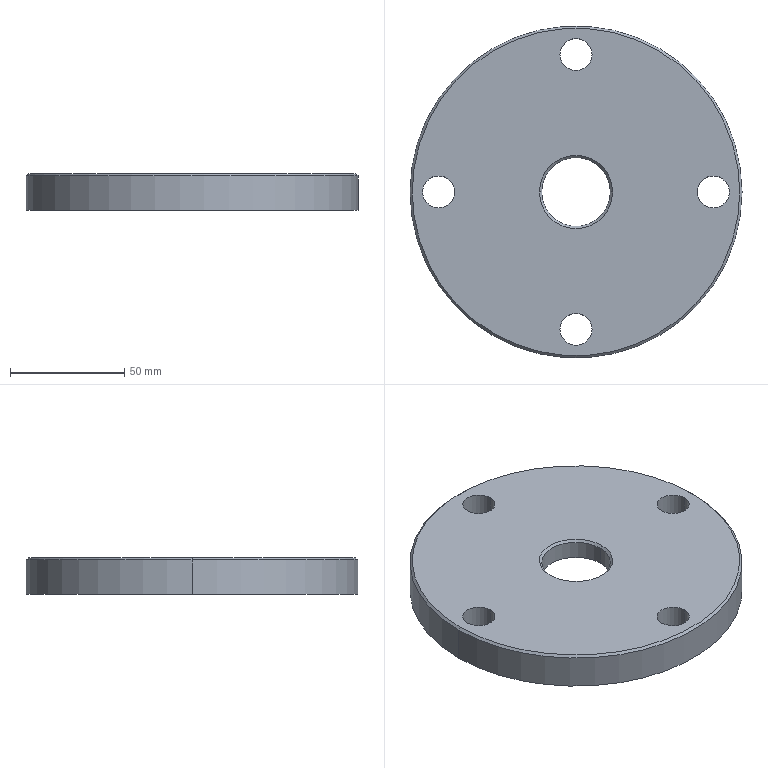Part | SolidWorks | features ICE 3, Chamfer 1, Extrusion 1 | 1 solid | 23 faces | box 145 x 145 x 16 mm | volume 201040 mm3 | cylinder 14 | cone 6 | plane 3 | commonest cylinder face diameters 14 x8 30 x2 92 x2 145 x2
STEP:
#1=CARTESIAN_POINT('',(71.5,0.,16.));
#2=VERTEX_POINT('',#1);
#3=CARTESIAN_POINT('',(-71.5,0.,16.));
#4=VERTEX_POINT('',#3);
#5=CARTESIAN_POINT('',(0.,0.,16.));
#6=DIRECTION('',(0.,0.,1.));
#7=DIRECTION('',(1.,0.,0.));
#8=AXIS2_PLACEMENT_3D('',#5,#6,#7);
#9=CIRCLE('',#8,71.5);
#10=EDGE_CURVE('',#2,#4,#9,.T.);
#11=ORIENTED_EDGE('',*,*,#10,.F.);
#12=CARTESIAN_POINT('',(72.5,0.,15.));
#13=VERTEX_POINT('',#12);
#14=CARTESIAN_POINT('',(71.5,0.,16.));
#15=DIRECTION('',(0.7071,0.,-0.7071));
#16=VECTOR('',#15,1000.);
#17=LINE('',#14,#16);
#18=EDGE_CURVE('',#2,#13,#17,.T.);
#19=ORIENTED_EDGE('',*,*,#18,.T.);
#20=CARTESIAN_POINT('',(-72.5,0.,15.));
#21=VERTEX_POINT('',#20);
#22=CARTESIAN_POINT('',(0.,0.,15.));
#23=DIRECTION('',(0.,0.,-1.));
#24=DIRECTION('',(1.,0.,0.));
#25=AXIS2_PLACEMENT_3D('',#22,#23,#24);
#26=CIRCLE('',#25,72.5);
#27=EDGE_CURVE('',#21,#13,#26,.T.);
#28=ORIENTED_EDGE('',*,*,#27,.F.);
#29=CARTESIAN_POINT('',(-71.5,0.,16.));
#30=DIRECTION('',(-0.7071,0.,-0.7071));
#31=VECTOR('',#30,1000.);
#32=LINE('',#29,#31);
#33=EDGE_CURVE('',#4,#21,#32,.T.);
#34=ORIENTED_EDGE('',*,*,#33,.F.);
#35=EDGE_LOOP('',(#11,#19,#28,#34));
#36=FACE_OUTER_BOUND('',#35,.T.);
#37=CARTESIAN_POINT('',(0.,0.,16.));
#38=DIRECTION('',(0.,0.,-1.));
#39=DIRECTION('',(-1.,0.,0.));
#40=AXIS2_PLACEMENT_3D('',#37,#38,#39);
#41=CONICAL_SURFACE('',#40,71.5,0.7854);
#42=ADVANCED_FACE('',(#36),#41,.T.);
#43=CARTESIAN_POINT('',(46.,0.,1.));
#44=VERTEX_POINT('',#43);
#45=CARTESIAN_POINT('',(-46.,0.,1.));
#46=VERTEX_POINT('',#45);
#47=CARTESIAN_POINT('',(0.,0.,1.));
#48=DIRECTION('',(0.,0.,-1.));
#49=DIRECTION('',(1.,0.,0.));
#50=AXIS2_PLACEMENT_3D('',#47,#48,#49);
#51=CIRCLE('',#50,46.);
#52=EDGE_CURVE('',#44,#46,#51,.T.);
#53=ORIENTED_EDGE('',*,*,#52,.F.);
#54=CARTESIAN_POINT('',(47.,0.,0.));
#55=VERTEX_POINT('',#54);
#56=CARTESIAN_POINT('',(46.,0.,1.));
#57=DIRECTION('',(0.7071,0.,-0.7071));
#58=VECTOR('',#57,1000.);
#59=LINE('',#56,#58);
#60=EDGE_CURVE('',#44,#55,#59,.T.);
#61=ORIENTED_EDGE('',*,*,#60,.T.);
#62=CARTESIAN_POINT('',(-47.,0.,0.));
#63=VERTEX_POINT('',#62);
#64=CARTESIAN_POINT('',(0.,0.,0.));
#65=DIRECTION('',(0.,0.,1.));
#66=DIRECTION('',(1.,0.,0.));
#67=AXIS2_PLACEMENT_3D('',#64,#65,#66);
#68=CIRCLE('',#67,47.);
#69=EDGE_CURVE('',#63,#55,#68,.T.);
#70=ORIENTED_EDGE('',*,*,#69,.F.);
#71=CARTESIAN_POINT('',(-46.,0.,1.));
#72=DIRECTION('',(-0.7071,0.,-0.7071));
#73=VECTOR('',#72,1000.);
#74=LINE('',#71,#73);
#75=EDGE_CURVE('',#46,#63,#74,.T.);
#76=ORIENTED_EDGE('',*,*,#75,.F.);
#77=EDGE_LOOP('',(#53,#61,#70,#76));
#78=FACE_OUTER_BOUND('',#77,.T.);
#79=CARTESIAN_POINT('',(0.,0.,1.));
#80=DIRECTION('',(0.,0.,-1.));
#81=DIRECTION('',(-1.,0.,0.));
#82=AXIS2_PLACEMENT_3D('',#79,#80,#81);
#83=CONICAL_SURFACE('',#82,46.,0.7854);
#84=ADVANCED_FACE('',(#78),#83,.F.);
#85=CARTESIAN_POINT('',(-15.,0.,15.));
#86=VERTEX_POINT('',#85);
#87=CARTESIAN_POINT('',(15.,0.,15.));
#88=VERTEX_POINT('',#87);
#89=CARTESIAN_POINT('',(0.,0.,15.));
#90=DIRECTION('',(0.,0.,1.));
#91=DIRECTION('',(1.,0.,0.));
#92=AXIS2_PLACEMENT_3D('',#89,#90,#91);
#93=CIRCLE('',#92,15.);
#94=EDGE_CURVE('',#86,#88,#93,.T.);
#95=ORIENTED_EDGE('',*,*,#94,.F.);
#96=CARTESIAN_POINT('',(-16.,0.,16.));
#97=VERTEX_POINT('',#96);
#98=CARTESIAN_POINT('',(-15.,0.,15.));
#99=DIRECTION('',(-0.7071,0.,0.7071));
#100=VECTOR('',#99,1000.);
#101=LINE('',#98,#100);
#102=EDGE_CURVE('',#86,#97,#101,.T.);
#103=ORIENTED_EDGE('',*,*,#102,.T.);
#104=CARTESIAN_POINT('',(16.,0.,16.));
#105=VERTEX_POINT('',#104);
#106=CARTESIAN_POINT('',(0.,0.,16.));
#107=DIRECTION('',(0.,0.,-1.));
#108=DIRECTION('',(1.,0.,0.));
#109=AXIS2_PLACEMENT_3D('',#106,#107,#108);
#110=CIRCLE('',#109,16.);
#111=EDGE_CURVE('',#105,#97,#110,.T.);
#112=ORIENTED_EDGE('',*,*,#111,.F.);
#113=CARTESIAN_POINT('',(15.,0.,15.));
#114=DIRECTION('',(0.7071,0.,0.7071));
#115=VECTOR('',#114,1000.);
#116=LINE('',#113,#115);
#117=EDGE_CURVE('',#88,#105,#116,.T.);
#118=ORIENTED_EDGE('',*,*,#117,.F.);
#119=EDGE_LOOP('',(#95,#103,#112,#118));
#120=FACE_OUTER_BOUND('',#119,.T.);
#121=CARTESIAN_POINT('',(0.,0.,15.));
#122=DIRECTION('',(0.,0.,1.));
#123=DIRECTION('',(1.,0.,0.));
#124=AXIS2_PLACEMENT_3D('',#121,#122,#123);
#125=CONICAL_SURFACE('',#124,15.,0.7854);
#126=ADVANCED_FACE('',(#120),#125,.F.);
#127=CARTESIAN_POINT('',(15.,0.,7.));
#128=VERTEX_POINT('',#127);
#129=CARTESIAN_POINT('',(-15.,0.,7.));
#130=VERTEX_POINT('',#129);
#131=CARTESIAN_POINT('',(0.,0.,7.));
#132=DIRECTION('',(0.,0.,-1.));
#133=DIRECTION('',(-1.,0.,0.));
#134=AXIS2_PLACEMENT_3D('',#131,#132,#133);
#135=CIRCLE('',#134,15.);
#136=EDGE_CURVE('',#128,#130,#135,.T.);
#137=ORIENTED_EDGE('',*,*,#136,.T.);
#138=CARTESIAN_POINT('',(-15.,0.,0.));
#139=DIRECTION('',(0.,0.,1.));
#140=VECTOR('',#139,1000.);
#141=LINE('',#138,#140);
#142=EDGE_CURVE('',#130,#86,#141,.T.);
#143=ORIENTED_EDGE('',*,*,#142,.T.);
#144=ORIENTED_EDGE('',*,*,#94,.T.);
#145=CARTESIAN_POINT('',(15.,0.,0.));
#146=DIRECTION('',(0.,0.,1.));
#147=VECTOR('',#146,1000.);
#148=LINE('',#145,#147);
#149=EDGE_CURVE('',#128,#88,#148,.T.);
#150=ORIENTED_EDGE('',*,*,#149,.F.);
#151=EDGE_LOOP('',(#137,#143,#144,#150));
#152=FACE_OUTER_BOUND('',#151,.T.);
#153=CARTESIAN_POINT('',(0.,0.,0.));
#154=DIRECTION('',(0.,0.,1.));
#155=DIRECTION('',(1.,0.,0.));
#156=AXIS2_PLACEMENT_3D('',#153,#154,#155);
#157=CYLINDRICAL_SURFACE('',#156,15.);
#158=ADVANCED_FACE('',(#152),#157,.F.);
#159=CARTESIAN_POINT('',(46.,0.,7.));
#160=VERTEX_POINT('',#159);
#161=CARTESIAN_POINT('',(-46.,0.,7.));
#162=VERTEX_POINT('',#161);
#163=CARTESIAN_POINT('',(0.,0.,7.));
#164=DIRECTION('',(0.,0.,-1.));
#165=DIRECTION('',(-1.,0.,0.));
#166=AXIS2_PLACEMENT_3D('',#163,#164,#165);
#167=CIRCLE('',#166,46.);
#168=EDGE_CURVE('',#160,#162,#167,.T.);
#169=ORIENTED_EDGE('',*,*,#168,.F.);
#170=CARTESIAN_POINT('',(46.,0.,7.));
#171=DIRECTION('',(0.,0.,-1.));
#172=VECTOR('',#171,1000.);
#173=LINE('',#170,#172);
#174=EDGE_CURVE('',#160,#44,#173,.T.);
#175=ORIENTED_EDGE('',*,*,#174,.T.);
#176=ORIENTED_EDGE('',*,*,#52,.T.);
#177=CARTESIAN_POINT('',(-46.,0.,7.));
#178=DIRECTION('',(0.,0.,-1.));
#179=VECTOR('',#178,1000.);
#180=LINE('',#177,#179);
#181=EDGE_CURVE('',#162,#46,#180,.T.);
#182=ORIENTED_EDGE('',*,*,#181,.F.);
#183=EDGE_LOOP('',(#169,#175,#176,#182));
#184=FACE_OUTER_BOUND('',#183,.T.);
#185=CARTESIAN_POINT('',(0.,0.,7.));
#186=DIRECTION('',(0.,0.,-1.));
#187=DIRECTION('',(-1.,0.,0.));
#188=AXIS2_PLACEMENT_3D('',#185,#186,#187);
#189=CYLINDRICAL_SURFACE('',#188,46.);
#190=ADVANCED_FACE('',(#184),#189,.F.);
#191=CARTESIAN_POINT('',(53.,0.,0.));
#192=VERTEX_POINT('',#191);
#193=CARTESIAN_POINT('',(67.,0.,0.));
#194=VERTEX_POINT('',#193);
#195=CARTESIAN_POINT('',(60.,0.,0.));
#196=DIRECTION('',(0.,0.,1.));
#197=DIRECTION('',(1.,0.,0.));
#198=AXIS2_PLACEMENT_3D('',#195,#196,#197);
#199=CIRCLE('',#198,7.);
#200=EDGE_CURVE('',#192,#194,#199,.T.);
#201=ORIENTED_EDGE('',*,*,#200,.F.);
#202=CARTESIAN_POINT('',(53.,0.,16.));
#203=VERTEX_POINT('',#202);
#204=CARTESIAN_POINT('',(53.,0.,0.));
#205=DIRECTION('',(0.,0.,1.));
#206=VECTOR('',#205,1000.);
#207=LINE('',#204,#206);
#208=EDGE_CURVE('',#192,#203,#207,.T.);
#209=ORIENTED_EDGE('',*,*,#208,.T.);
#210=CARTESIAN_POINT('',(67.,0.,16.));
#211=VERTEX_POINT('',#210);
#212=CARTESIAN_POINT('',(60.,0.,16.));
#213=DIRECTION('',(0.,0.,1.));
#214=DIRECTION('',(1.,0.,0.));
#215=AXIS2_PLACEMENT_3D('',#212,#213,#214);
#216=CIRCLE('',#215,7.);
#217=EDGE_CURVE('',#203,#211,#216,.T.);
#218=ORIENTED_EDGE('',*,*,#217,.T.);
#219=CARTESIAN_POINT('',(67.,0.,0.));
#220=DIRECTION('',(0.,0.,1.));
#221=VECTOR('',#220,1000.);
#222=LINE('',#219,#221);
#223=EDGE_CURVE('',#194,#211,#222,.T.);
#224=ORIENTED_EDGE('',*,*,#223,.F.);
#225=EDGE_LOOP('',(#201,#209,#218,#224));
#226=FACE_OUTER_BOUND('',#225,.T.);
#227=CARTESIAN_POINT('',(60.,0.,0.));
#228=DIRECTION('',(0.,0.,1.));
#229=DIRECTION('',(1.,0.,0.));
#230=AXIS2_PLACEMENT_3D('',#227,#228,#229);
#231=CYLINDRICAL_SURFACE('',#230,7.);
#232=ADVANCED_FACE('',(#226),#231,.F.);
#233=CARTESIAN_POINT('',(-7.,-60.,0.));
#234=VERTEX_POINT('',#233);
#235=CARTESIAN_POINT('',(7.,-60.,0.));
#236=VERTEX_POINT('',#235);
#237=CARTESIAN_POINT('',(0.,-60.,0.));
#238=DIRECTION('',(0.,0.,1.));
#239=DIRECTION('',(1.,0.,0.));
#240=AXIS2_PLACEMENT_3D('',#237,#238,#239);
#241=CIRCLE('',#240,7.);
#242=EDGE_CURVE('',#234,#236,#241,.T.);
#243=ORIENTED_EDGE('',*,*,#242,.F.);
#244=CARTESIAN_POINT('',(-7.,-60.,16.));
#245=VERTEX_POINT('',#244);
#246=CARTESIAN_POINT('',(-7.,-60.,0.));
#247=DIRECTION('',(0.,0.,1.));
#248=VECTOR('',#247,1000.);
#249=LINE('',#246,#248);
#250=EDGE_CURVE('',#234,#245,#249,.T.);
#251=ORIENTED_EDGE('',*,*,#250,.T.);
#252=CARTESIAN_POINT('',(7.,-60.,16.));
#253=VERTEX_POINT('',#252);
#254=CARTESIAN_POINT('',(0.,-60.,16.));
#255=DIRECTION('',(0.,0.,1.));
#256=DIRECTION('',(1.,0.,0.));
#257=AXIS2_PLACEMENT_3D('',#254,#255,#256);
#258=CIRCLE('',#257,7.);
#259=EDGE_CURVE('',#245,#253,#258,.T.);
#260=ORIENTED_EDGE('',*,*,#259,.T.);
#261=CARTESIAN_POINT('',(7.,-60.,0.));
#262=DIRECTION('',(0.,0.,1.));
#263=VECTOR('',#262,1000.);
#264=LINE('',#261,#263);
#265=EDGE_CURVE('',#236,#253,#264,.T.);
#266=ORIENTED_EDGE('',*,*,#265,.F.);
#267=EDGE_LOOP('',(#243,#251,#260,#266));
#268=FACE_OUTER_BOUND('',#267,.T.);
#269=CARTESIAN_POINT('',(0.,-60.,0.));
#270=DIRECTION('',(0.,0.,1.));
#271=DIRECTION('',(1.,0.,0.));
#272=AXIS2_PLACEMENT_3D('',#269,#270,#271);
#273=CYLINDRICAL_SURFACE('',#272,7.);
#274=ADVANCED_FACE('',(#268),#273,.F.);
#275=CARTESIAN_POINT('',(-67.,0.,0.));
#276=VERTEX_POINT('',#275);
#277=CARTESIAN_POINT('',(-53.,0.,0.));
#278=VERTEX_POINT('',#277);
#279=CARTESIAN_POINT('',(-60.,0.,0.));
#280=DIRECTION('',(0.,0.,1.));
#281=DIRECTION('',(1.,0.,0.));
#282=AXIS2_PLACEMENT_3D('',#279,#280,#281);
#283=CIRCLE('',#282,7.);
#284=EDGE_CURVE('',#276,#278,#283,.T.);
#285=ORIENTED_EDGE('',*,*,#284,.F.);
#286=CARTESIAN_POINT('',(-67.,0.,16.));
#287=VERTEX_POINT('',#286);
#288=CARTESIAN_POINT('',(-67.,0.,0.));
#289=DIRECTION('',(0.,0.,1.));
#290=VECTOR('',#289,1000.);
#291=LINE('',#288,#290);
#292=EDGE_CURVE('',#276,#287,#291,.T.);
#293=ORIENTED_EDGE('',*,*,#292,.T.);
#294=CARTESIAN_POINT('',(-53.,0.,16.));
#295=VERTEX_POINT('',#294);
#296=CARTESIAN_POINT('',(-60.,0.,16.));
#297=DIRECTION('',(0.,0.,1.));
#298=DIRECTION('',(1.,0.,0.));
#299=AXIS2_PLACEMENT_3D('',#296,#297,#298);
#300=CIRCLE('',#299,7.);
#301=EDGE_CURVE('',#287,#295,#300,.T.);
#302=ORIENTED_EDGE('',*,*,#301,.T.);
#303=CARTESIAN_POINT('',(-53.,0.,0.));
#304=DIRECTION('',(0.,0.,1.));
#305=VECTOR('',#304,1000.);
#306=LINE('',#303,#305);
#307=EDGE_CURVE('',#278,#295,#306,.T.);
#308=ORIENTED_EDGE('',*,*,#307,.F.);
#309=EDGE_LOOP('',(#285,#293,#302,#308));
#310=FACE_OUTER_BOUND('',#309,.T.);
#311=CARTESIAN_POINT('',(-60.,0.,0.));
#312=DIRECTION('',(0.,0.,1.));
#313=DIRECTION('',(1.,0.,0.));
#314=AXIS2_PLACEMENT_3D('',#311,#312,#313);
#315=CYLINDRICAL_SURFACE('',#314,7.);
#316=ADVANCED_FACE('',(#310),#315,.F.);
#317=CARTESIAN_POINT('',(-7.,60.,0.));
#318=VERTEX_POINT('',#317);
#319=CARTESIAN_POINT('',(7.,60.,0.));
#320=VERTEX_POINT('',#319);
#321=CARTESIAN_POINT('',(0.,60.,0.));
#322=DIRECTION('',(0.,0.,1.));
#323=DIRECTION('',(1.,0.,0.));
#324=AXIS2_PLACEMENT_3D('',#321,#322,#323);
#325=CIRCLE('',#324,7.);
#326=EDGE_CURVE('',#318,#320,#325,.T.);
#327=ORIENTED_EDGE('',*,*,#326,.F.);
#328=CARTESIAN_POINT('',(-7.,60.,16.));
#329=VERTEX_POINT('',#328);
#330=CARTESIAN_POINT('',(-7.,60.,0.));
#331=DIRECTION('',(0.,0.,1.));
#332=VECTOR('',#331,1000.);
#333=LINE('',#330,#332);
#334=EDGE_CURVE('',#318,#329,#333,.T.);
#335=ORIENTED_EDGE('',*,*,#334,.T.);
#336=CARTESIAN_POINT('',(7.,60.,16.));
#337=VERTEX_POINT('',#336);
#338=CARTESIAN_POINT('',(0.,60.,16.));
#339=DIRECTION('',(0.,0.,1.));
#340=DIRECTION('',(1.,0.,0.));
#341=AXIS2_PLACEMENT_3D('',#338,#339,#340);
#342=CIRCLE('',#341,7.);
#343=EDGE_CURVE('',#329,#337,#342,.T.);
#344=ORIENTED_EDGE('',*,*,#343,.T.);
#345=CARTESIAN_POINT('',(7.,60.,0.));
#346=DIRECTION('',(0.,0.,1.));
#347=VECTOR('',#346,1000.);
#348=LINE('',#345,#347);
#349=EDGE_CURVE('',#320,#337,#348,.T.);
#350=ORIENTED_EDGE('',*,*,#349,.F.);
#351=EDGE_LOOP('',(#327,#335,#344,#350));
#352=FACE_OUTER_BOUND('',#351,.T.);
#353=CARTESIAN_POINT('',(0.,60.,0.));
#354=DIRECTION('',(0.,0.,1.));
#355=DIRECTION('',(1.,0.,0.));
#356=AXIS2_PLACEMENT_3D('',#353,#354,#355);
#357=CYLINDRICAL_SURFACE('',#356,7.);
#358=ADVANCED_FACE('',(#352),#357,.F.);
#359=ORIENTED_EDGE('',*,*,#27,.T.);
#360=CARTESIAN_POINT('',(72.5,0.,0.));
#361=VERTEX_POINT('',#360);
#362=CARTESIAN_POINT('',(72.5,0.,16.));
#363=DIRECTION('',(0.,0.,-1.));
#364=VECTOR('',#363,1000.);
#365=LINE('',#362,#364);
#366=EDGE_CURVE('',#13,#361,#365,.T.);
#367=ORIENTED_EDGE('',*,*,#366,.T.);
#368=CARTESIAN_POINT('',(-72.5,0.,0.));
#369=VERTEX_POINT('',#368);
#370=CARTESIAN_POINT('',(0.,0.,0.));
#371=DIRECTION('',(0.,0.,1.));
#372=DIRECTION('',(1.,0.,0.));
#373=AXIS2_PLACEMENT_3D('',#370,#371,#372);
#374=CIRCLE('',#373,72.5);
#375=EDGE_CURVE('',#361,#369,#374,.T.);
#376=ORIENTED_EDGE('',*,*,#375,.T.);
#377=CARTESIAN_POINT('',(-72.5,0.,16.));
#378=DIRECTION('',(0.,0.,-1.));
#379=VECTOR('',#378,1000.);
#380=LINE('',#377,#379);
#381=EDGE_CURVE('',#21,#369,#380,.T.);
#382=ORIENTED_EDGE('',*,*,#381,.F.);
#383=EDGE_LOOP('',(#359,#367,#376,#382));
#384=FACE_OUTER_BOUND('',#383,.T.);
#385=CARTESIAN_POINT('',(0.,0.,16.));
#386=DIRECTION('',(0.,0.,-1.));
#387=DIRECTION('',(-1.,0.,0.));
#388=AXIS2_PLACEMENT_3D('',#385,#386,#387);
#389=CYLINDRICAL_SURFACE('',#388,72.5);
#390=ADVANCED_FACE('',(#384),#389,.T.);
#391=ORIENTED_EDGE('',*,*,#366,.F.);
#392=CARTESIAN_POINT('',(0.,0.,15.));
#393=DIRECTION('',(0.,0.,-1.));
#394=DIRECTION('',(1.,0.,0.));
#395=AXIS2_PLACEMENT_3D('',#392,#393,#394);
#396=CIRCLE('',#395,72.5);
#397=EDGE_CURVE('',#13,#21,#396,.T.);
#398=ORIENTED_EDGE('',*,*,#397,.T.);
#399=ORIENTED_EDGE('',*,*,#381,.T.);
#400=CARTESIAN_POINT('',(0.,0.,0.));
#401=DIRECTION('',(0.,0.,1.));
#402=DIRECTION('',(1.,0.,0.));
#403=AXIS2_PLACEMENT_3D('',#400,#401,#402);
#404=CIRCLE('',#403,72.5);
#405=EDGE_CURVE('',#369,#361,#404,.T.);
#406=ORIENTED_EDGE('',*,*,#405,.T.);
#407=EDGE_LOOP('',(#391,#398,#399,#406));
#408=FACE_OUTER_BOUND('',#407,.T.);
#409=CARTESIAN_POINT('',(0.,0.,16.));
#410=DIRECTION('',(0.,0.,-1.));
#411=DIRECTION('',(-1.,0.,0.));
#412=AXIS2_PLACEMENT_3D('',#409,#410,#411);
#413=CYLINDRICAL_SURFACE('',#412,72.5);
#414=ADVANCED_FACE('',(#408),#413,.T.);
#415=ORIENTED_EDGE('',*,*,#111,.T.);
#416=CARTESIAN_POINT('',(0.,0.,16.));
#417=DIRECTION('',(0.,0.,-1.));
#418=DIRECTION('',(1.,0.,0.));
#419=AXIS2_PLACEMENT_3D('',#416,#417,#418);
#420=CIRCLE('',#419,16.);
#421=EDGE_CURVE('',#97,#105,#420,.T.);
#422=ORIENTED_EDGE('',*,*,#421,.T.);
#423=EDGE_LOOP('',(#415,#422));
#424=FACE_BOUND('',#423,.T.);
#425=CARTESIAN_POINT('',(0.,0.,16.));
#426=DIRECTION('',(0.,0.,1.));
#427=DIRECTION('',(1.,0.,0.));
#428=AXIS2_PLACEMENT_3D('',#425,#426,#427);
#429=CIRCLE('',#428,71.5);
#430=EDGE_CURVE('',#4,#2,#429,.T.);
#431=ORIENTED_EDGE('',*,*,#430,.T.);
#432=ORIENTED_EDGE('',*,*,#10,.T.);
#433=EDGE_LOOP('',(#431,#432));
#434=FACE_OUTER_BOUND('',#433,.T.);
#435=CARTESIAN_POINT('',(60.,0.,16.));
#436=DIRECTION('',(0.,0.,1.));
#437=DIRECTION('',(1.,0.,0.));
#438=AXIS2_PLACEMENT_3D('',#435,#436,#437);
#439=CIRCLE('',#438,7.);
#440=EDGE_CURVE('',#211,#203,#439,.T.);
#441=ORIENTED_EDGE('',*,*,#440,.F.);
#442=ORIENTED_EDGE('',*,*,#217,.F.);
#443=EDGE_LOOP('',(#441,#442));
#444=FACE_BOUND('',#443,.T.);
#445=CARTESIAN_POINT('',(0.,-60.,16.));
#446=DIRECTION('',(0.,0.,1.));
#447=DIRECTION('',(1.,0.,0.));
#448=AXIS2_PLACEMENT_3D('',#445,#446,#447);
#449=CIRCLE('',#448,7.);
#450=EDGE_CURVE('',#253,#245,#449,.T.);
#451=ORIENTED_EDGE('',*,*,#450,.F.);
#452=ORIENTED_EDGE('',*,*,#259,.F.);
#453=EDGE_LOOP('',(#451,#452));
#454=FACE_BOUND('',#453,.T.);
#455=CARTESIAN_POINT('',(-60.,0.,16.));
#456=DIRECTION('',(0.,0.,1.));
#457=DIRECTION('',(1.,0.,0.));
#458=AXIS2_PLACEMENT_3D('',#455,#456,#457);
#459=CIRCLE('',#458,7.);
#460=EDGE_CURVE('',#295,#287,#459,.T.);
#461=ORIENTED_EDGE('',*,*,#460,.F.);
#462=ORIENTED_EDGE('',*,*,#301,.F.);
#463=EDGE_LOOP('',(#461,#462));
#464=FACE_BOUND('',#463,.T.);
#465=CARTESIAN_POINT('',(0.,60.,16.));
#466=DIRECTION('',(0.,0.,1.));
#467=DIRECTION('',(1.,0.,0.));
#468=AXIS2_PLACEMENT_3D('',#465,#466,#467);
#469=CIRCLE('',#468,7.);
#470=EDGE_CURVE('',#337,#329,#469,.T.);
#471=ORIENTED_EDGE('',*,*,#470,.F.);
#472=ORIENTED_EDGE('',*,*,#343,.F.);
#473=EDGE_LOOP('',(#471,#472));
#474=FACE_BOUND('',#473,.T.);
#475=CARTESIAN_POINT('',(0.,0.,16.));
#476=DIRECTION('',(0.,0.,1.));
#477=DIRECTION('',(1.,0.,0.));
#478=AXIS2_PLACEMENT_3D('',#475,#476,#477);
#479=PLANE('',#478);
#480=ADVANCED_FACE('',(#424,#434,#444,#454,#464,#474),#479,.T.);
#481=ORIENTED_EDGE('',*,*,#69,.T.);
#482=CARTESIAN_POINT('',(0.,0.,0.));
#483=DIRECTION('',(0.,0.,1.));
#484=DIRECTION('',(1.,0.,0.));
#485=AXIS2_PLACEMENT_3D('',#482,#483,#484);
#486=CIRCLE('',#485,47.);
#487=EDGE_CURVE('',#55,#63,#486,.T.);
#488=ORIENTED_EDGE('',*,*,#487,.T.);
#489=EDGE_LOOP('',(#481,#488));
#490=FACE_BOUND('',#489,.T.);
#491=CARTESIAN_POINT('',(60.,0.,0.));
#492=DIRECTION('',(0.,0.,1.));
#493=DIRECTION('',(1.,0.,0.));
#494=AXIS2_PLACEMENT_3D('',#491,#492,#493);
#495=CIRCLE('',#494,7.);
#496=EDGE_CURVE('',#194,#192,#495,.T.);
#497=ORIENTED_EDGE('',*,*,#496,.T.);
#498=ORIENTED_EDGE('',*,*,#200,.T.);
#499=EDGE_LOOP('',(#497,#498));
#500=FACE_BOUND('',#499,.T.);
#501=CARTESIAN_POINT('',(0.,-60.,0.));
#502=DIRECTION('',(0.,0.,1.));
#503=DIRECTION('',(1.,0.,0.));
#504=AXIS2_PLACEMENT_3D('',#501,#502,#503);
#505=CIRCLE('',#504,7.);
#506=EDGE_CURVE('',#236,#234,#505,.T.);
#507=ORIENTED_EDGE('',*,*,#506,.T.);
#508=ORIENTED_EDGE('',*,*,#242,.T.);
#509=EDGE_LOOP('',(#507,#508));
#510=FACE_BOUND('',#509,.T.);
#511=CARTESIAN_POINT('',(-60.,0.,0.));
#512=DIRECTION('',(0.,0.,1.));
#513=DIRECTION('',(1.,0.,0.));
#514=AXIS2_PLACEMENT_3D('',#511,#512,#513);
#515=CIRCLE('',#514,7.);
#516=EDGE_CURVE('',#278,#276,#515,.T.);
#517=ORIENTED_EDGE('',*,*,#516,.T.);
#518=ORIENTED_EDGE('',*,*,#284,.T.);
#519=EDGE_LOOP('',(#517,#518));
#520=FACE_BOUND('',#519,.T.);
#521=CARTESIAN_POINT('',(0.,60.,0.));
#522=DIRECTION('',(0.,0.,1.));
#523=DIRECTION('',(1.,0.,0.));
#524=AXIS2_PLACEMENT_3D('',#521,#522,#523);
#525=CIRCLE('',#524,7.);
#526=EDGE_CURVE('',#320,#318,#525,.T.);
#527=ORIENTED_EDGE('',*,*,#526,.T.);
#528=ORIENTED_EDGE('',*,*,#326,.T.);
#529=EDGE_LOOP('',(#527,#528));
#530=FACE_BOUND('',#529,.T.);
#531=ORIENTED_EDGE('',*,*,#405,.F.);
#532=ORIENTED_EDGE('',*,*,#375,.F.);
#533=EDGE_LOOP('',(#531,#532));
#534=FACE_OUTER_BOUND('',#533,.T.);
#535=CARTESIAN_POINT('',(0.,0.,0.));
#536=DIRECTION('',(0.,0.,1.));
#537=DIRECTION('',(1.,0.,0.));
#538=AXIS2_PLACEMENT_3D('',#535,#536,#537);
#539=PLANE('',#538);
#540=ADVANCED_FACE('',(#490,#500,#510,#520,#530,#534),#539,.F.);
#541=ORIENTED_EDGE('',*,*,#334,.F.);
#542=ORIENTED_EDGE('',*,*,#526,.F.);
#543=ORIENTED_EDGE('',*,*,#349,.T.);
#544=ORIENTED_EDGE('',*,*,#470,.T.);
#545=EDGE_LOOP('',(#541,#542,#543,#544));
#546=FACE_OUTER_BOUND('',#545,.T.);
#547=CARTESIAN_POINT('',(0.,60.,0.));
#548=DIRECTION('',(0.,0.,1.));
#549=DIRECTION('',(1.,0.,0.));
#550=AXIS2_PLACEMENT_3D('',#547,#548,#549);
#551=CYLINDRICAL_SURFACE('',#550,7.);
#552=ADVANCED_FACE('',(#546),#551,.F.);
#553=ORIENTED_EDGE('',*,*,#292,.F.);
#554=ORIENTED_EDGE('',*,*,#516,.F.);
#555=ORIENTED_EDGE('',*,*,#307,.T.);
#556=ORIENTED_EDGE('',*,*,#460,.T.);
#557=EDGE_LOOP('',(#553,#554,#555,#556));
#558=FACE_OUTER_BOUND('',#557,.T.);
#559=CARTESIAN_POINT('',(-60.,0.,0.));
#560=DIRECTION('',(0.,0.,1.));
#561=DIRECTION('',(1.,0.,0.));
#562=AXIS2_PLACEMENT_3D('',#559,#560,#561);
#563=CYLINDRICAL_SURFACE('',#562,7.);
#564=ADVANCED_FACE('',(#558),#563,.F.);
#565=ORIENTED_EDGE('',*,*,#250,.F.);
#566=ORIENTED_EDGE('',*,*,#506,.F.);
#567=ORIENTED_EDGE('',*,*,#265,.T.);
#568=ORIENTED_EDGE('',*,*,#450,.T.);
#569=EDGE_LOOP('',(#565,#566,#567,#568));
#570=FACE_OUTER_BOUND('',#569,.T.);
#571=CARTESIAN_POINT('',(0.,-60.,0.));
#572=DIRECTION('',(0.,0.,1.));
#573=DIRECTION('',(1.,0.,0.));
#574=AXIS2_PLACEMENT_3D('',#571,#572,#573);
#575=CYLINDRICAL_SURFACE('',#574,7.);
#576=ADVANCED_FACE('',(#570),#575,.F.);
#577=ORIENTED_EDGE('',*,*,#208,.F.);
#578=ORIENTED_EDGE('',*,*,#496,.F.);
#579=ORIENTED_EDGE('',*,*,#223,.T.);
#580=ORIENTED_EDGE('',*,*,#440,.T.);
#581=EDGE_LOOP('',(#577,#578,#579,#580));
#582=FACE_OUTER_BOUND('',#581,.T.);
#583=CARTESIAN_POINT('',(60.,0.,0.));
#584=DIRECTION('',(0.,0.,1.));
#585=DIRECTION('',(1.,0.,0.));
#586=AXIS2_PLACEMENT_3D('',#583,#584,#585);
#587=CYLINDRICAL_SURFACE('',#586,7.);
#588=ADVANCED_FACE('',(#582),#587,.F.);
#589=ORIENTED_EDGE('',*,*,#174,.F.);
#590=CARTESIAN_POINT('',(0.,0.,7.));
#591=DIRECTION('',(0.,0.,-1.));
#592=DIRECTION('',(-1.,0.,0.));
#593=AXIS2_PLACEMENT_3D('',#590,#591,#592);
#594=CIRCLE('',#593,46.);
#595=EDGE_CURVE('',#162,#160,#594,.T.);
#596=ORIENTED_EDGE('',*,*,#595,.F.);
#597=ORIENTED_EDGE('',*,*,#181,.T.);
#598=CARTESIAN_POINT('',(0.,0.,1.));
#599=DIRECTION('',(0.,0.,-1.));
#600=DIRECTION('',(1.,0.,0.));
#601=AXIS2_PLACEMENT_3D('',#598,#599,#600);
#602=CIRCLE('',#601,46.);
#603=EDGE_CURVE('',#46,#44,#602,.T.);
#604=ORIENTED_EDGE('',*,*,#603,.T.);
#605=EDGE_LOOP('',(#589,#596,#597,#604));
#606=FACE_OUTER_BOUND('',#605,.T.);
#607=CARTESIAN_POINT('',(0.,0.,7.));
#608=DIRECTION('',(0.,0.,-1.));
#609=DIRECTION('',(-1.,0.,0.));
#610=AXIS2_PLACEMENT_3D('',#607,#608,#609);
#611=CYLINDRICAL_SURFACE('',#610,46.);
#612=ADVANCED_FACE('',(#606),#611,.F.);
#613=ORIENTED_EDGE('',*,*,#136,.F.);
#614=CARTESIAN_POINT('',(0.,0.,7.));
#615=DIRECTION('',(0.,0.,-1.));
#616=DIRECTION('',(-1.,0.,0.));
#617=AXIS2_PLACEMENT_3D('',#614,#615,#616);
#618=CIRCLE('',#617,15.);
#619=EDGE_CURVE('',#130,#128,#618,.T.);
#620=ORIENTED_EDGE('',*,*,#619,.F.);
#621=EDGE_LOOP('',(#613,#620));
#622=FACE_BOUND('',#621,.T.);
#623=ORIENTED_EDGE('',*,*,#595,.T.);
#624=ORIENTED_EDGE('',*,*,#168,.T.);
#625=EDGE_LOOP('',(#623,#624));
#626=FACE_OUTER_BOUND('',#625,.T.);
#627=CARTESIAN_POINT('',(0.,0.,7.));
#628=DIRECTION('',(0.,0.,-1.));
#629=DIRECTION('',(-1.,0.,0.));
#630=AXIS2_PLACEMENT_3D('',#627,#628,#629);
#631=PLANE('',#630);
#632=ADVANCED_FACE('',(#622,#626),#631,.T.);
#633=ORIENTED_EDGE('',*,*,#142,.F.);
#634=ORIENTED_EDGE('',*,*,#619,.T.);
#635=ORIENTED_EDGE('',*,*,#149,.T.);
#636=CARTESIAN_POINT('',(0.,0.,15.));
#637=DIRECTION('',(0.,0.,1.));
#638=DIRECTION('',(1.,0.,0.));
#639=AXIS2_PLACEMENT_3D('',#636,#637,#638);
#640=CIRCLE('',#639,15.);
#641=EDGE_CURVE('',#88,#86,#640,.T.);
#642=ORIENTED_EDGE('',*,*,#641,.T.);
#643=EDGE_LOOP('',(#633,#634,#635,#642));
#644=FACE_OUTER_BOUND('',#643,.T.);
#645=CARTESIAN_POINT('',(0.,0.,0.));
#646=DIRECTION('',(0.,0.,1.));
#647=DIRECTION('',(1.,0.,0.));
#648=AXIS2_PLACEMENT_3D('',#645,#646,#647);
#649=CYLINDRICAL_SURFACE('',#648,15.);
#650=ADVANCED_FACE('',(#644),#649,.F.);
#651=ORIENTED_EDGE('',*,*,#102,.F.);
#652=ORIENTED_EDGE('',*,*,#641,.F.);
#653=ORIENTED_EDGE('',*,*,#117,.T.);
#654=ORIENTED_EDGE('',*,*,#421,.F.);
#655=EDGE_LOOP('',(#651,#652,#653,#654));
#656=FACE_OUTER_BOUND('',#655,.T.);
#657=CARTESIAN_POINT('',(0.,0.,15.));
#658=DIRECTION('',(0.,0.,1.));
#659=DIRECTION('',(1.,0.,0.));
#660=AXIS2_PLACEMENT_3D('',#657,#658,#659);
#661=CONICAL_SURFACE('',#660,15.,0.7854);
#662=ADVANCED_FACE('',(#656),#661,.F.);
#663=ORIENTED_EDGE('',*,*,#60,.F.);
#664=ORIENTED_EDGE('',*,*,#603,.F.);
#665=ORIENTED_EDGE('',*,*,#75,.T.);
#666=ORIENTED_EDGE('',*,*,#487,.F.);
#667=EDGE_LOOP('',(#663,#664,#665,#666));
#668=FACE_OUTER_BOUND('',#667,.T.);
#669=CARTESIAN_POINT('',(0.,0.,1.));
#670=DIRECTION('',(0.,0.,-1.));
#671=DIRECTION('',(-1.,0.,0.));
#672=AXIS2_PLACEMENT_3D('',#669,#670,#671);
#673=CONICAL_SURFACE('',#672,46.,0.7854);
#674=ADVANCED_FACE('',(#668),#673,.F.);
#675=ORIENTED_EDGE('',*,*,#18,.F.);
#676=ORIENTED_EDGE('',*,*,#430,.F.);
#677=ORIENTED_EDGE('',*,*,#33,.T.);
#678=ORIENTED_EDGE('',*,*,#397,.F.);
#679=EDGE_LOOP('',(#675,#676,#677,#678));
#680=FACE_OUTER_BOUND('',#679,.T.);
#681=CARTESIAN_POINT('',(0.,0.,16.));
#682=DIRECTION('',(0.,0.,-1.));
#683=DIRECTION('',(-1.,0.,0.));
#684=AXIS2_PLACEMENT_3D('',#681,#682,#683);
#685=CONICAL_SURFACE('',#684,71.5,0.7854);
#686=ADVANCED_FACE('',(#680),#685,.T.);
#687=CLOSED_SHELL('',(#42,#84,#126,#158,#190,#232,#274,#316,#358,#390,#414,#480,#540,#552,#564,#576,#588,#612,#632,#650,#662,#674,#686));
#688=MANIFOLD_SOLID_BREP('',#687);
#689=CARTESIAN_POINT('',(0.,0.,0.));
#690=DIRECTION('',(0.,0.,1.));
#691=DIRECTION('',(1.,0.,0.));
#692=AXIS2_PLACEMENT_3D('',#689,#690,#691);
#693=(LENGTH_UNIT()NAMED_UNIT(*)SI_UNIT(.MILLI.,.METRE.));
#694=UNCERTAINTY_MEASURE_WITH_UNIT(LENGTH_MEASURE(0.00001),#693,'','');
#695=(NAMED_UNIT(*)PLANE_ANGLE_UNIT()SI_UNIT($,.RADIAN.));
#696=(NAMED_UNIT(*)SI_UNIT($,.STERADIAN.)SOLID_ANGLE_UNIT());
#697=(GEOMETRIC_REPRESENTATION_CONTEXT(3)GLOBAL_UNCERTAINTY_ASSIGNED_CONTEXT((#694))GLOBAL_UNIT_ASSIGNED_CONTEXT((#693,#695,#696))REPRESENTATION_CONTEXT('',''));
#698=ADVANCED_BREP_SHAPE_REPRESENTATION('',(#688,#692),#697);